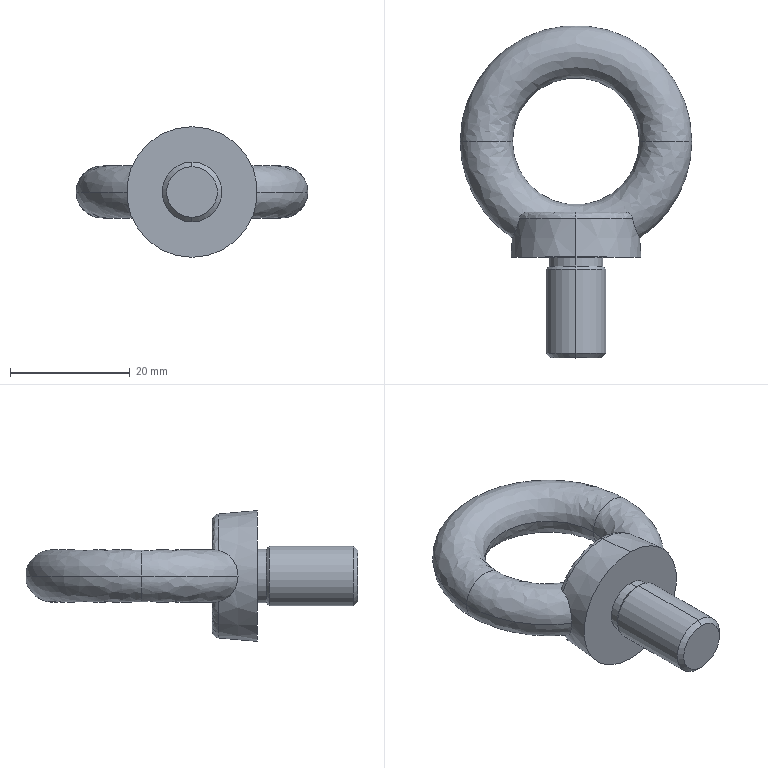Part | STEP file | Part 65 | 1 solid | 21 faces | box 38.75 x 55.625 x 21.875 mm | volume 8627 mm3 | spline 7 | cone 6 | cylinder 4 | plane 4 | commonest cylinder face diameters 9 x2 10 x2